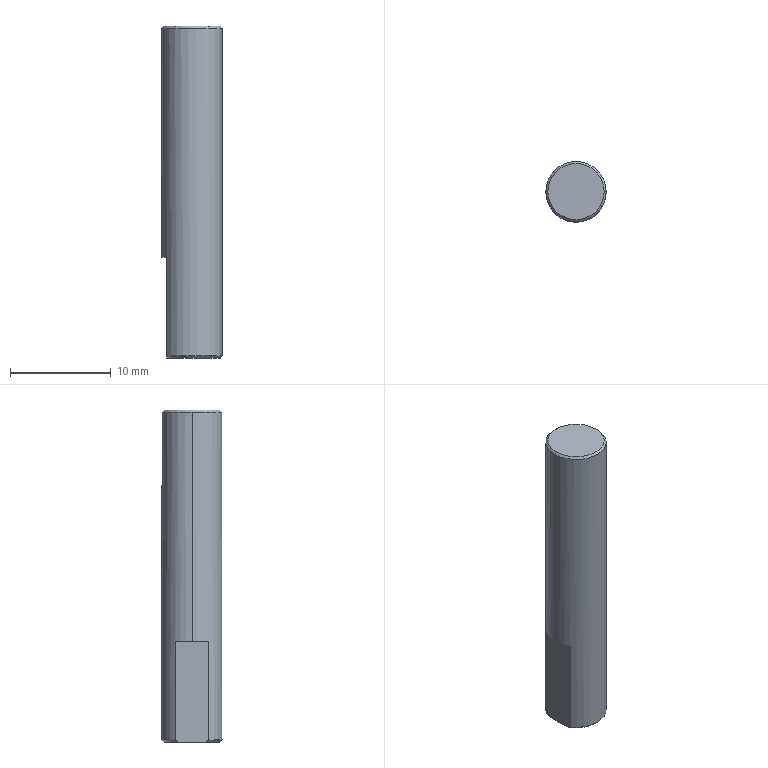Part | SolidWorks | features Chamfer 1, Extrusion 1, ICE 1 | 1 solid | 10 faces | box 6 x 6 x 33 mm | volume 921.126 mm3 | cone 4 | plane 4 | cylinder 2 | commonest cylinder face diameters 6 x2
STEP:
#1=CARTESIAN_POINT('',(2.8,0.,16.5));
#2=VERTEX_POINT('',#1);
#3=CARTESIAN_POINT('',(-2.8,0.,16.5));
#4=VERTEX_POINT('',#3);
#5=CARTESIAN_POINT('',(0.,0.,16.5));
#6=DIRECTION('',(0.,0.,1.));
#7=DIRECTION('',(1.,0.,0.));
#8=AXIS2_PLACEMENT_3D('',#5,#6,#7);
#9=CIRCLE('',#8,2.8);
#10=EDGE_CURVE('',#2,#4,#9,.T.);
#11=ORIENTED_EDGE('',*,*,#10,.F.);
#12=CARTESIAN_POINT('',(3.,0.,16.3));
#13=VERTEX_POINT('',#12);
#14=CARTESIAN_POINT('',(2.8,0.,16.5));
#15=DIRECTION('',(0.7071,0.,-0.7071));
#16=VECTOR('',#15,1000.);
#17=LINE('',#14,#16);
#18=EDGE_CURVE('',#2,#13,#17,.T.);
#19=ORIENTED_EDGE('',*,*,#18,.T.);
#20=CARTESIAN_POINT('',(-3.,0.,16.3));
#21=VERTEX_POINT('',#20);
#22=CARTESIAN_POINT('',(0.,0.,16.3));
#23=DIRECTION('',(0.,0.,-1.));
#24=DIRECTION('',(1.,0.,0.));
#25=AXIS2_PLACEMENT_3D('',#22,#23,#24);
#26=CIRCLE('',#25,3.);
#27=EDGE_CURVE('',#21,#13,#26,.T.);
#28=ORIENTED_EDGE('',*,*,#27,.F.);
#29=CARTESIAN_POINT('',(-2.8,0.,16.5));
#30=DIRECTION('',(-0.7071,0.,-0.7071));
#31=VECTOR('',#30,1000.);
#32=LINE('',#29,#31);
#33=EDGE_CURVE('',#4,#21,#32,.T.);
#34=ORIENTED_EDGE('',*,*,#33,.F.);
#35=EDGE_LOOP('',(#11,#19,#28,#34));
#36=FACE_OUTER_BOUND('',#35,.T.);
#37=CARTESIAN_POINT('',(0.,0.,16.5));
#38=DIRECTION('',(0.,0.,-1.));
#39=DIRECTION('',(-1.,0.,0.));
#40=AXIS2_PLACEMENT_3D('',#37,#38,#39);
#41=CONICAL_SURFACE('',#40,2.8,0.7854);
#42=ADVANCED_FACE('',(#36),#41,.T.);
#43=CARTESIAN_POINT('',(2.8,0.,-16.5));
#44=VERTEX_POINT('',#43);
#45=CARTESIAN_POINT('',(-2.5,-1.261,-16.5));
#46=VERTEX_POINT('',#45);
#47=CARTESIAN_POINT('',(0.,0.,-16.5));
#48=DIRECTION('',(0.,0.,-1.));
#49=DIRECTION('',(1.,0.,0.));
#50=AXIS2_PLACEMENT_3D('',#47,#48,#49);
#51=CIRCLE('',#50,2.8);
#52=EDGE_CURVE('',#44,#46,#51,.T.);
#53=ORIENTED_EDGE('',*,*,#52,.F.);
#54=CARTESIAN_POINT('',(3.,0.,-16.3));
#55=VERTEX_POINT('',#54);
#56=CARTESIAN_POINT('',(3.,0.,-16.3));
#57=DIRECTION('',(0.7071,0.,0.7071));
#58=VECTOR('',#57,1000.);
#59=LINE('',#56,#58);
#60=EDGE_CURVE('',#44,#55,#59,.T.);
#61=ORIENTED_EDGE('',*,*,#60,.T.);
#62=CARTESIAN_POINT('',(-2.5,-1.658,-16.3));
#63=VERTEX_POINT('',#62);
#64=CARTESIAN_POINT('',(0.,0.,-16.3));
#65=DIRECTION('',(0.,0.,1.));
#66=DIRECTION('',(1.,0.,0.));
#67=AXIS2_PLACEMENT_3D('',#64,#65,#66);
#68=CIRCLE('',#67,3.);
#69=EDGE_CURVE('',#63,#55,#68,.T.);
#70=ORIENTED_EDGE('',*,*,#69,.F.);
#71=CARTESIAN_POINT('',(-2.5,-1.261,-16.5));
#72=CARTESIAN_POINT('',(-2.5,-1.397,-16.439));
#73=CARTESIAN_POINT('',(-2.5,-1.529,-16.372));
#74=CARTESIAN_POINT('',(-2.5,-1.658,-16.3));
#75=B_SPLINE_CURVE_WITH_KNOTS('',3,(#71,#72,#73,#74),.UNSPECIFIED.,.F.,.F.,(4,4),(0.008797,0.009246),.UNSPECIFIED.);
#76=EDGE_CURVE('',#46,#63,#75,.T.);
#77=ORIENTED_EDGE('',*,*,#76,.F.);
#78=EDGE_LOOP('',(#53,#61,#70,#77));
#79=FACE_OUTER_BOUND('',#78,.T.);
#80=CARTESIAN_POINT('',(0.,0.,-16.3));
#81=DIRECTION('',(0.,0.,1.));
#82=DIRECTION('',(1.,0.,0.));
#83=AXIS2_PLACEMENT_3D('',#80,#81,#82);
#84=CONICAL_SURFACE('',#83,3.,0.7854);
#85=ADVANCED_FACE('',(#79),#84,.T.);
#86=ORIENTED_EDGE('',*,*,#27,.T.);
#87=CARTESIAN_POINT('',(3.,0.,16.5));
#88=DIRECTION('',(0.,0.,-1.));
#89=VECTOR('',#88,1000.);
#90=LINE('',#87,#89);
#91=EDGE_CURVE('',#13,#55,#90,.T.);
#92=ORIENTED_EDGE('',*,*,#91,.T.);
#93=CARTESIAN_POINT('',(-2.5,1.658,-16.3));
#94=VERTEX_POINT('',#93);
#95=CARTESIAN_POINT('',(0.,0.,-16.3));
#96=DIRECTION('',(0.,0.,1.));
#97=DIRECTION('',(1.,0.,0.));
#98=AXIS2_PLACEMENT_3D('',#95,#96,#97);
#99=CIRCLE('',#98,3.);
#100=EDGE_CURVE('',#55,#94,#99,.T.);
#101=ORIENTED_EDGE('',*,*,#100,.T.);
#102=CARTESIAN_POINT('',(-2.5,1.658,-6.5));
#103=VERTEX_POINT('',#102);
#104=CARTESIAN_POINT('',(-2.5,1.658,16.5));
#105=DIRECTION('',(0.,0.,1.));
#106=VECTOR('',#105,1000.);
#107=LINE('',#104,#106);
#108=EDGE_CURVE('',#94,#103,#107,.T.);
#109=ORIENTED_EDGE('',*,*,#108,.T.);
#110=CARTESIAN_POINT('',(-3.,0.,-6.5));
#111=VERTEX_POINT('',#110);
#112=CARTESIAN_POINT('',(0.,0.,-6.5));
#113=DIRECTION('',(0.,0.,1.));
#114=DIRECTION('',(1.,0.,0.));
#115=AXIS2_PLACEMENT_3D('',#112,#113,#114);
#116=CIRCLE('',#115,3.);
#117=EDGE_CURVE('',#103,#111,#116,.T.);
#118=ORIENTED_EDGE('',*,*,#117,.T.);
#119=CARTESIAN_POINT('',(-3.,0.,16.5));
#120=DIRECTION('',(0.,0.,-1.));
#121=VECTOR('',#120,1000.);
#122=LINE('',#119,#121);
#123=EDGE_CURVE('',#21,#111,#122,.T.);
#124=ORIENTED_EDGE('',*,*,#123,.F.);
#125=EDGE_LOOP('',(#86,#92,#101,#109,#118,#124));
#126=FACE_OUTER_BOUND('',#125,.T.);
#127=CARTESIAN_POINT('',(0.,0.,16.5));
#128=DIRECTION('',(0.,0.,-1.));
#129=DIRECTION('',(-1.,0.,0.));
#130=AXIS2_PLACEMENT_3D('',#127,#128,#129);
#131=CYLINDRICAL_SURFACE('',#130,3.);
#132=ADVANCED_FACE('',(#126),#131,.T.);
#133=ORIENTED_EDGE('',*,*,#91,.F.);
#134=CARTESIAN_POINT('',(0.,0.,16.3));
#135=DIRECTION('',(0.,0.,-1.));
#136=DIRECTION('',(1.,0.,0.));
#137=AXIS2_PLACEMENT_3D('',#134,#135,#136);
#138=CIRCLE('',#137,3.);
#139=EDGE_CURVE('',#13,#21,#138,.T.);
#140=ORIENTED_EDGE('',*,*,#139,.T.);
#141=ORIENTED_EDGE('',*,*,#123,.T.);
#142=CARTESIAN_POINT('',(-2.5,-1.658,-6.5));
#143=VERTEX_POINT('',#142);
#144=CARTESIAN_POINT('',(0.,0.,-6.5));
#145=DIRECTION('',(0.,0.,1.));
#146=DIRECTION('',(1.,0.,0.));
#147=AXIS2_PLACEMENT_3D('',#144,#145,#146);
#148=CIRCLE('',#147,3.);
#149=EDGE_CURVE('',#111,#143,#148,.T.);
#150=ORIENTED_EDGE('',*,*,#149,.T.);
#151=CARTESIAN_POINT('',(-2.5,-1.658,16.5));
#152=DIRECTION('',(0.,0.,-1.));
#153=VECTOR('',#152,1000.);
#154=LINE('',#151,#153);
#155=EDGE_CURVE('',#143,#63,#154,.T.);
#156=ORIENTED_EDGE('',*,*,#155,.T.);
#157=ORIENTED_EDGE('',*,*,#69,.T.);
#158=EDGE_LOOP('',(#133,#140,#141,#150,#156,#157));
#159=FACE_OUTER_BOUND('',#158,.T.);
#160=CARTESIAN_POINT('',(0.,0.,16.5));
#161=DIRECTION('',(0.,0.,-1.));
#162=DIRECTION('',(-1.,0.,0.));
#163=AXIS2_PLACEMENT_3D('',#160,#161,#162);
#164=CYLINDRICAL_SURFACE('',#163,3.);
#165=ADVANCED_FACE('',(#159),#164,.T.);
#166=CARTESIAN_POINT('',(0.,0.,16.5));
#167=DIRECTION('',(0.,0.,1.));
#168=DIRECTION('',(1.,0.,0.));
#169=AXIS2_PLACEMENT_3D('',#166,#167,#168);
#170=CIRCLE('',#169,2.8);
#171=EDGE_CURVE('',#4,#2,#170,.T.);
#172=ORIENTED_EDGE('',*,*,#171,.T.);
#173=ORIENTED_EDGE('',*,*,#10,.T.);
#174=EDGE_LOOP('',(#172,#173));
#175=FACE_OUTER_BOUND('',#174,.T.);
#176=CARTESIAN_POINT('',(0.,0.,16.5));
#177=DIRECTION('',(0.,0.,1.));
#178=DIRECTION('',(1.,0.,0.));
#179=AXIS2_PLACEMENT_3D('',#176,#177,#178);
#180=PLANE('',#179);
#181=ADVANCED_FACE('',(#175),#180,.T.);
#182=CARTESIAN_POINT('',(-2.5,1.261,-16.5));
#183=VERTEX_POINT('',#182);
#184=CARTESIAN_POINT('',(0.,0.,-16.5));
#185=DIRECTION('',(0.,0.,-1.));
#186=DIRECTION('',(1.,0.,0.));
#187=AXIS2_PLACEMENT_3D('',#184,#185,#186);
#188=CIRCLE('',#187,2.8);
#189=EDGE_CURVE('',#183,#44,#188,.T.);
#190=ORIENTED_EDGE('',*,*,#189,.T.);
#191=ORIENTED_EDGE('',*,*,#52,.T.);
#192=CARTESIAN_POINT('',(-2.5,-15.,-16.5));
#193=DIRECTION('',(0.,1.,0.));
#194=VECTOR('',#193,1000.);
#195=LINE('',#192,#194);
#196=EDGE_CURVE('',#46,#183,#195,.T.);
#197=ORIENTED_EDGE('',*,*,#196,.T.);
#198=EDGE_LOOP('',(#190,#191,#197));
#199=FACE_OUTER_BOUND('',#198,.T.);
#200=CARTESIAN_POINT('',(0.,0.,-16.5));
#201=DIRECTION('',(0.,0.,1.));
#202=DIRECTION('',(1.,0.,0.));
#203=AXIS2_PLACEMENT_3D('',#200,#201,#202);
#204=PLANE('',#203);
#205=ADVANCED_FACE('',(#199),#204,.F.);
#206=ORIENTED_EDGE('',*,*,#60,.F.);
#207=ORIENTED_EDGE('',*,*,#189,.F.);
#208=CARTESIAN_POINT('',(-2.5,1.658,-16.3));
#209=CARTESIAN_POINT('',(-2.5,1.528,-16.372));
#210=CARTESIAN_POINT('',(-2.5,1.396,-16.439));
#211=CARTESIAN_POINT('',(-2.5,1.261,-16.5));
#212=B_SPLINE_CURVE_WITH_KNOTS('',3,(#208,#209,#210,#211),.UNSPECIFIED.,.F.,.F.,(4,4),(0.005738,0.006184),.UNSPECIFIED.);
#213=EDGE_CURVE('',#94,#183,#212,.T.);
#214=ORIENTED_EDGE('',*,*,#213,.F.);
#215=ORIENTED_EDGE('',*,*,#100,.F.);
#216=EDGE_LOOP('',(#206,#207,#214,#215));
#217=FACE_OUTER_BOUND('',#216,.T.);
#218=CARTESIAN_POINT('',(0.,0.,-16.3));
#219=DIRECTION('',(0.,0.,1.));
#220=DIRECTION('',(1.,0.,0.));
#221=AXIS2_PLACEMENT_3D('',#218,#219,#220);
#222=CONICAL_SURFACE('',#221,3.,0.7854);
#223=ADVANCED_FACE('',(#217),#222,.T.);
#224=ORIENTED_EDGE('',*,*,#18,.F.);
#225=ORIENTED_EDGE('',*,*,#171,.F.);
#226=ORIENTED_EDGE('',*,*,#33,.T.);
#227=ORIENTED_EDGE('',*,*,#139,.F.);
#228=EDGE_LOOP('',(#224,#225,#226,#227));
#229=FACE_OUTER_BOUND('',#228,.T.);
#230=CARTESIAN_POINT('',(0.,0.,16.5));
#231=DIRECTION('',(0.,0.,-1.));
#232=DIRECTION('',(-1.,0.,0.));
#233=AXIS2_PLACEMENT_3D('',#230,#231,#232);
#234=CONICAL_SURFACE('',#233,2.8,0.7854);
#235=ADVANCED_FACE('',(#229),#234,.T.);
#236=CARTESIAN_POINT('',(-2.5,-15.,-6.5));
#237=DIRECTION('',(0.,1.,0.));
#238=VECTOR('',#237,1000.);
#239=LINE('',#236,#238);
#240=EDGE_CURVE('',#143,#103,#239,.T.);
#241=ORIENTED_EDGE('',*,*,#240,.F.);
#242=ORIENTED_EDGE('',*,*,#149,.F.);
#243=ORIENTED_EDGE('',*,*,#117,.F.);
#244=EDGE_LOOP('',(#241,#242,#243));
#245=FACE_OUTER_BOUND('',#244,.T.);
#246=CARTESIAN_POINT('',(-3.,-15.,-6.5));
#247=DIRECTION('',(0.,0.,1.));
#248=DIRECTION('',(1.,0.,0.));
#249=AXIS2_PLACEMENT_3D('',#246,#247,#248);
#250=PLANE('',#249);
#251=ADVANCED_FACE('',(#245),#250,.F.);
#252=ORIENTED_EDGE('',*,*,#213,.T.);
#253=ORIENTED_EDGE('',*,*,#196,.F.);
#254=ORIENTED_EDGE('',*,*,#76,.T.);
#255=ORIENTED_EDGE('',*,*,#155,.F.);
#256=ORIENTED_EDGE('',*,*,#240,.T.);
#257=ORIENTED_EDGE('',*,*,#108,.F.);
#258=EDGE_LOOP('',(#252,#253,#254,#255,#256,#257));
#259=FACE_OUTER_BOUND('',#258,.T.);
#260=CARTESIAN_POINT('',(-2.5,-15.,-16.5));
#261=DIRECTION('',(1.,0.,0.));
#262=DIRECTION('',(0.,0.,-1.));
#263=AXIS2_PLACEMENT_3D('',#260,#261,#262);
#264=PLANE('',#263);
#265=ADVANCED_FACE('',(#259),#264,.F.);
#266=CLOSED_SHELL('',(#42,#85,#132,#165,#181,#205,#223,#235,#251,#265));
#267=MANIFOLD_SOLID_BREP('',#266);
#268=CARTESIAN_POINT('',(0.,0.,0.));
#269=DIRECTION('',(0.,0.,1.));
#270=DIRECTION('',(1.,0.,0.));
#271=AXIS2_PLACEMENT_3D('',#268,#269,#270);
#272=(LENGTH_UNIT()NAMED_UNIT(*)SI_UNIT(.MILLI.,.METRE.));
#273=UNCERTAINTY_MEASURE_WITH_UNIT(LENGTH_MEASURE(0.00001),#272,'','');
#274=(NAMED_UNIT(*)PLANE_ANGLE_UNIT()SI_UNIT($,.RADIAN.));
#275=(NAMED_UNIT(*)SI_UNIT($,.STERADIAN.)SOLID_ANGLE_UNIT());
#276=(GEOMETRIC_REPRESENTATION_CONTEXT(3)GLOBAL_UNCERTAINTY_ASSIGNED_CONTEXT((#273))GLOBAL_UNIT_ASSIGNED_CONTEXT((#272,#274,#275))REPRESENTATION_CONTEXT('',''));
#277=ADVANCED_BREP_SHAPE_REPRESENTATION('',(#267,#271),#276);